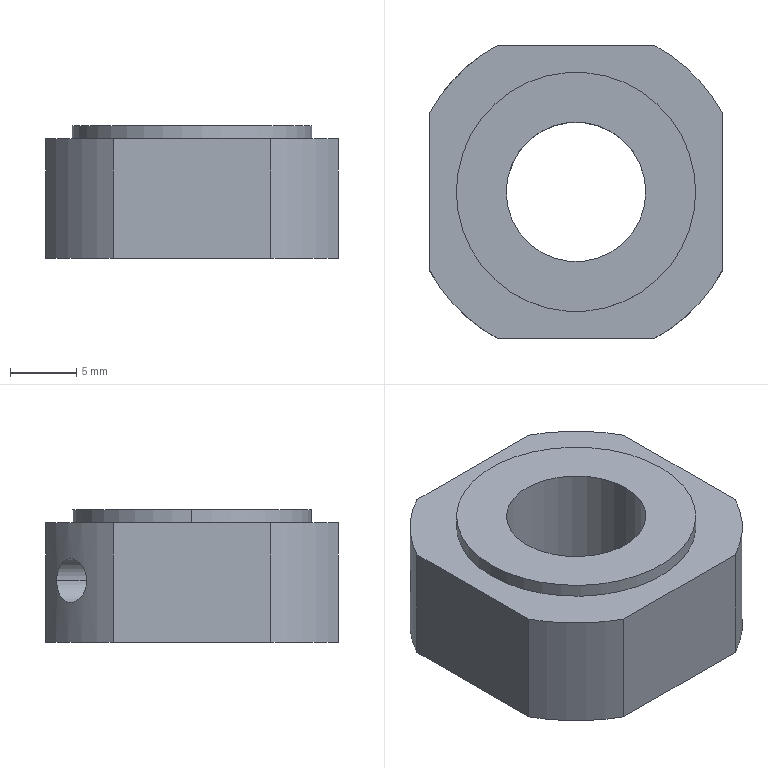Part | SolidWorks | features HoleWzd 2, 3DProfileFeature 1, Extrusion 1, ICE 1 | 1 solid | 17 faces | box 22 x 22 x 10 mm | volume 3311 mm3 | cylinder 10 | plane 7 | commonest cylinder face diameters 25 x4 3.3 x2 10.5 x2 18 x2
STEP:
#1=CARTESIAN_POINT('',(-5.25,0.,0.));
#2=VERTEX_POINT('',#1);
#3=CARTESIAN_POINT('',(5.25,0.,0.));
#4=VERTEX_POINT('',#3);
#5=CARTESIAN_POINT('',(0.,0.,0.));
#6=DIRECTION('',(0.,0.,1.));
#7=DIRECTION('',(1.,0.,0.));
#8=AXIS2_PLACEMENT_3D('',#5,#6,#7);
#9=CIRCLE('',#8,5.25);
#10=EDGE_CURVE('',#2,#4,#9,.T.);
#11=ORIENTED_EDGE('',*,*,#10,.F.);
#12=CARTESIAN_POINT('',(-5.25,0.,10.));
#13=VERTEX_POINT('',#12);
#14=CARTESIAN_POINT('',(-5.25,0.,10.));
#15=DIRECTION('',(0.,0.,1.));
#16=VECTOR('',#15,1000.);
#17=LINE('',#14,#16);
#18=EDGE_CURVE('',#2,#13,#17,.T.);
#19=ORIENTED_EDGE('',*,*,#18,.T.);
#20=CARTESIAN_POINT('',(5.25,0.,10.));
#21=VERTEX_POINT('',#20);
#22=CARTESIAN_POINT('',(0.,0.,10.));
#23=DIRECTION('',(0.,0.,1.));
#24=DIRECTION('',(1.,0.,0.));
#25=AXIS2_PLACEMENT_3D('',#22,#23,#24);
#26=CIRCLE('',#25,5.25);
#27=EDGE_CURVE('',#13,#21,#26,.T.);
#28=ORIENTED_EDGE('',*,*,#27,.T.);
#29=CARTESIAN_POINT('',(5.25,0.,10.));
#30=DIRECTION('',(0.,0.,1.));
#31=VECTOR('',#30,1000.);
#32=LINE('',#29,#31);
#33=EDGE_CURVE('',#4,#21,#32,.T.);
#34=ORIENTED_EDGE('',*,*,#33,.F.);
#35=EDGE_LOOP('',(#11,#19,#28,#34));
#36=FACE_OUTER_BOUND('',#35,.T.);
#37=CARTESIAN_POINT('',(0.,0.,10.));
#38=DIRECTION('',(0.,0.,1.));
#39=DIRECTION('',(1.,0.,0.));
#40=AXIS2_PLACEMENT_3D('',#37,#38,#39);
#41=CYLINDRICAL_SURFACE('',#40,5.25);
#42=ADVANCED_FACE('',(#36),#41,.F.);
#43=CARTESIAN_POINT('',(-4.609,2.514,4.65));
#44=VERTEX_POINT('',#43);
#45=CARTESIAN_POINT('',(-2.198,4.768,4.65));
#46=VERTEX_POINT('',#45);
#47=CARTESIAN_POINT('',(-4.609,2.514,4.65));
#48=CARTESIAN_POINT('',(-4.609,2.514,4.54));
#49=CARTESIAN_POINT('',(-4.603,2.525,4.432));
#50=CARTESIAN_POINT('',(-4.582,2.563,4.22));
#51=CARTESIAN_POINT('',(-4.565,2.593,4.115));
#52=CARTESIAN_POINT('',(-4.522,2.668,3.916));
#53=CARTESIAN_POINT('',(-4.495,2.713,3.821));
#54=CARTESIAN_POINT('',(-4.429,2.819,3.642));
#55=CARTESIAN_POINT('',(-4.391,2.879,3.558));
#56=CARTESIAN_POINT('',(-4.261,3.072,3.332));
#57=CARTESIAN_POINT('',(-4.15,3.221,3.209));
#58=CARTESIAN_POINT('',(-3.958,3.451,3.085));
#59=CARTESIAN_POINT('',(-3.888,3.53,3.053));
#60=CARTESIAN_POINT('',(-3.741,3.685,3.01));
#61=CARTESIAN_POINT('',(-3.665,3.761,3.));
#62=CARTESIAN_POINT('',(-3.506,3.909,3.));
#63=CARTESIAN_POINT('',(-3.423,3.982,3.01));
#64=CARTESIAN_POINT('',(-3.259,4.117,3.053));
#65=CARTESIAN_POINT('',(-3.177,4.181,3.084));
#66=CARTESIAN_POINT('',(-2.932,4.359,3.21));
#67=CARTESIAN_POINT('',(-2.777,4.458,3.331));
#68=CARTESIAN_POINT('',(-2.575,4.576,3.56));
#69=CARTESIAN_POINT('',(-2.514,4.61,3.642));
#70=CARTESIAN_POINT('',(-2.404,4.667,3.82));
#71=CARTESIAN_POINT('',(-2.356,4.692,3.917));
#72=CARTESIAN_POINT('',(-2.279,4.73,4.116));
#73=CARTESIAN_POINT('',(-2.249,4.744,4.219));
#74=CARTESIAN_POINT('',(-2.208,4.763,4.432));
#75=CARTESIAN_POINT('',(-2.198,4.768,4.541));
#76=CARTESIAN_POINT('',(-2.198,4.768,4.65));
#77=B_SPLINE_CURVE_WITH_KNOTS('',3,(#47,#48,#49,#50,#51,#52,#53,#54,#55,#56,#57,#58,#59,#60,#61,#62,#63,#64,#65,#66,#67,#68,#69,#70,#71,#72,#73,#74,#75,#76),.UNSPECIFIED.,.F.,.F.,(4,2,2,2,2,2,2,2,2,2,2,2,2,2,4),(0.,0.0003245,0.000649,0.0009734,0.001298,0.001947,0.002271,0.002596,0.00292,0.003245,0.003894,0.004218,0.004543,0.004867,0.005192),.UNSPECIFIED.);
#78=EDGE_CURVE('',#44,#46,#77,.T.);
#79=ORIENTED_EDGE('',*,*,#78,.T.);
#80=CARTESIAN_POINT('',(-7.255,10.179,4.65));
#81=VERTEX_POINT('',#80);
#82=CARTESIAN_POINT('',(-7.33,10.259,4.65));
#83=DIRECTION('',(-0.6828,0.7306,0.));
#84=VECTOR('',#83,1000.);
#85=LINE('',#82,#84);
#86=EDGE_CURVE('',#46,#81,#85,.T.);
#87=ORIENTED_EDGE('',*,*,#86,.T.);
#88=CARTESIAN_POINT('',(-9.666,7.926,4.65));
#89=VERTEX_POINT('',#88);
#90=CARTESIAN_POINT('',(-9.666,7.926,4.65));
#91=CARTESIAN_POINT('',(-9.666,7.926,4.54));
#92=CARTESIAN_POINT('',(-9.659,7.934,4.433));
#93=CARTESIAN_POINT('',(-9.632,7.967,4.222));
#94=CARTESIAN_POINT('',(-9.612,7.991,4.117));
#95=CARTESIAN_POINT('',(-9.558,8.055,3.917));
#96=CARTESIAN_POINT('',(-9.525,8.094,3.823));
#97=CARTESIAN_POINT('',(-9.447,8.186,3.643));
#98=CARTESIAN_POINT('',(-9.401,8.239,3.559));
#99=CARTESIAN_POINT('',(-9.249,8.41,3.331));
#100=CARTESIAN_POINT('',(-9.124,8.546,3.208));
#101=CARTESIAN_POINT('',(-8.848,8.832,3.043));
#102=CARTESIAN_POINT('',(-8.693,8.985,3.));
#103=CARTESIAN_POINT('',(-8.457,9.205,3.));
#104=CARTESIAN_POINT('',(-8.376,9.279,3.01));
#105=CARTESIAN_POINT('',(-8.218,9.42,3.053));
#106=CARTESIAN_POINT('',(-8.14,9.487,3.084));
#107=CARTESIAN_POINT('',(-7.987,9.616,3.166));
#108=CARTESIAN_POINT('',(-7.912,9.677,3.218));
#109=CARTESIAN_POINT('',(-7.773,9.79,3.338));
#110=CARTESIAN_POINT('',(-7.707,9.842,3.406));
#111=CARTESIAN_POINT('',(-7.585,9.936,3.56));
#112=CARTESIAN_POINT('',(-7.53,9.978,3.643));
#113=CARTESIAN_POINT('',(-7.434,10.049,3.822));
#114=CARTESIAN_POINT('',(-7.392,10.08,3.918));
#115=CARTESIAN_POINT('',(-7.324,10.129,4.118));
#116=CARTESIAN_POINT('',(-7.299,10.148,4.221));
#117=CARTESIAN_POINT('',(-7.264,10.173,4.432));
#118=CARTESIAN_POINT('',(-7.255,10.179,4.542));
#119=CARTESIAN_POINT('',(-7.255,10.179,4.65));
#120=B_SPLINE_CURVE_WITH_KNOTS('',3,(#90,#91,#92,#93,#94,#95,#96,#97,#98,#99,#100,#101,#102,#103,#104,#105,#106,#107,#108,#109,#110,#111,#112,#113,#114,#115,#116,#117,#118,#119),.UNSPECIFIED.,.F.,.F.,(4,2,2,2,2,2,2,2,2,2,2,2,2,2,4),(0.,0.0003228,0.0006455,0.0009683,0.001291,0.001937,0.002582,0.002905,0.003228,0.00355,0.003873,0.004196,0.004519,0.004842,0.005164),.UNSPECIFIED.);
#121=EDGE_CURVE('',#89,#81,#120,.T.);
#122=ORIENTED_EDGE('',*,*,#121,.F.);
#123=CARTESIAN_POINT('',(-9.741,8.005,4.65));
#124=DIRECTION('',(-0.6828,0.7306,0.));
#125=VECTOR('',#124,1000.);
#126=LINE('',#123,#125);
#127=EDGE_CURVE('',#44,#89,#126,.T.);
#128=ORIENTED_EDGE('',*,*,#127,.F.);
#129=EDGE_LOOP('',(#79,#87,#122,#128));
#130=FACE_OUTER_BOUND('',#129,.T.);
#131=CARTESIAN_POINT('',(-8.535,9.132,4.65));
#132=DIRECTION('',(-0.6828,0.7306,0.));
#133=DIRECTION('',(-0.7306,-0.6828,0.));
#134=AXIS2_PLACEMENT_3D('',#131,#132,#133);
#135=CYLINDRICAL_SURFACE('',#134,1.65);
#136=ADVANCED_FACE('',(#130),#135,.F.);
#137=CARTESIAN_POINT('',(9.,0.,9.));
#138=VERTEX_POINT('',#137);
#139=CARTESIAN_POINT('',(-9.,0.,9.));
#140=VERTEX_POINT('',#139);
#141=CARTESIAN_POINT('',(0.,0.,9.));
#142=DIRECTION('',(0.,0.,1.));
#143=DIRECTION('',(1.,0.,0.));
#144=AXIS2_PLACEMENT_3D('',#141,#142,#143);
#145=CIRCLE('',#144,9.);
#146=EDGE_CURVE('',#138,#140,#145,.T.);
#147=ORIENTED_EDGE('',*,*,#146,.T.);
#148=CARTESIAN_POINT('',(-9.,0.,10.));
#149=VERTEX_POINT('',#148);
#150=CARTESIAN_POINT('',(-9.,0.,9.));
#151=DIRECTION('',(0.,0.,1.));
#152=VECTOR('',#151,1000.);
#153=LINE('',#150,#152);
#154=EDGE_CURVE('',#140,#149,#153,.T.);
#155=ORIENTED_EDGE('',*,*,#154,.T.);
#156=CARTESIAN_POINT('',(9.,0.,10.));
#157=VERTEX_POINT('',#156);
#158=CARTESIAN_POINT('',(0.,0.,10.));
#159=DIRECTION('',(0.,0.,1.));
#160=DIRECTION('',(1.,0.,0.));
#161=AXIS2_PLACEMENT_3D('',#158,#159,#160);
#162=CIRCLE('',#161,9.);
#163=EDGE_CURVE('',#157,#149,#162,.T.);
#164=ORIENTED_EDGE('',*,*,#163,.F.);
#165=CARTESIAN_POINT('',(9.,0.,9.));
#166=DIRECTION('',(0.,0.,1.));
#167=VECTOR('',#166,1000.);
#168=LINE('',#165,#167);
#169=EDGE_CURVE('',#138,#157,#168,.T.);
#170=ORIENTED_EDGE('',*,*,#169,.F.);
#171=EDGE_LOOP('',(#147,#155,#164,#170));
#172=FACE_OUTER_BOUND('',#171,.T.);
#173=CARTESIAN_POINT('',(0.,0.,9.));
#174=DIRECTION('',(0.,0.,1.));
#175=DIRECTION('',(1.,0.,0.));
#176=AXIS2_PLACEMENT_3D('',#173,#174,#175);
#177=CYLINDRICAL_SURFACE('',#176,9.);
#178=ADVANCED_FACE('',(#172),#177,.T.);
#179=CARTESIAN_POINT('',(5.937,-11.,9.));
#180=VERTEX_POINT('',#179);
#181=CARTESIAN_POINT('',(11.,-5.937,9.));
#182=VERTEX_POINT('',#181);
#183=CARTESIAN_POINT('',(0.,0.,9.));
#184=DIRECTION('',(0.,0.,1.));
#185=DIRECTION('',(1.,0.,0.));
#186=AXIS2_PLACEMENT_3D('',#183,#184,#185);
#187=CIRCLE('',#186,12.5);
#188=EDGE_CURVE('',#180,#182,#187,.T.);
#189=ORIENTED_EDGE('',*,*,#188,.F.);
#190=CARTESIAN_POINT('',(5.937,-11.,0.));
#191=VERTEX_POINT('',#190);
#192=CARTESIAN_POINT('',(5.937,-11.,10.));
#193=DIRECTION('',(0.,0.,-1.));
#194=VECTOR('',#193,1000.);
#195=LINE('',#192,#194);
#196=EDGE_CURVE('',#180,#191,#195,.T.);
#197=ORIENTED_EDGE('',*,*,#196,.T.);
#198=CARTESIAN_POINT('',(11.,-5.937,0.));
#199=VERTEX_POINT('',#198);
#200=CARTESIAN_POINT('',(0.,0.,0.));
#201=DIRECTION('',(0.,0.,1.));
#202=DIRECTION('',(1.,0.,0.));
#203=AXIS2_PLACEMENT_3D('',#200,#201,#202);
#204=CIRCLE('',#203,12.5);
#205=EDGE_CURVE('',#191,#199,#204,.T.);
#206=ORIENTED_EDGE('',*,*,#205,.T.);
#207=CARTESIAN_POINT('',(11.,-5.937,10.));
#208=DIRECTION('',(0.,0.,-1.));
#209=VECTOR('',#208,1000.);
#210=LINE('',#207,#209);
#211=EDGE_CURVE('',#182,#199,#210,.T.);
#212=ORIENTED_EDGE('',*,*,#211,.F.);
#213=EDGE_LOOP('',(#189,#197,#206,#212));
#214=FACE_OUTER_BOUND('',#213,.T.);
#215=CARTESIAN_POINT('',(0.,0.,10.));
#216=DIRECTION('',(0.,0.,-1.));
#217=DIRECTION('',(-1.,0.,0.));
#218=AXIS2_PLACEMENT_3D('',#215,#216,#217);
#219=CYLINDRICAL_SURFACE('',#218,12.5);
#220=ADVANCED_FACE('',(#214),#219,.T.);
#221=CARTESIAN_POINT('',(11.,5.937,9.));
#222=VERTEX_POINT('',#221);
#223=CARTESIAN_POINT('',(11.,-5.937,9.));
#224=DIRECTION('',(0.,1.,0.));
#225=VECTOR('',#224,1000.);
#226=LINE('',#223,#225);
#227=EDGE_CURVE('',#182,#222,#226,.T.);
#228=ORIENTED_EDGE('',*,*,#227,.F.);
#229=ORIENTED_EDGE('',*,*,#211,.T.);
#230=CARTESIAN_POINT('',(11.,5.937,0.));
#231=VERTEX_POINT('',#230);
#232=CARTESIAN_POINT('',(11.,-5.937,0.));
#233=DIRECTION('',(0.,1.,0.));
#234=VECTOR('',#233,1000.);
#235=LINE('',#232,#234);
#236=EDGE_CURVE('',#199,#231,#235,.T.);
#237=ORIENTED_EDGE('',*,*,#236,.T.);
#238=CARTESIAN_POINT('',(11.,5.937,10.));
#239=DIRECTION('',(0.,0.,-1.));
#240=VECTOR('',#239,1000.);
#241=LINE('',#238,#240);
#242=EDGE_CURVE('',#222,#231,#241,.T.);
#243=ORIENTED_EDGE('',*,*,#242,.F.);
#244=EDGE_LOOP('',(#228,#229,#237,#243));
#245=FACE_OUTER_BOUND('',#244,.T.);
#246=CARTESIAN_POINT('',(11.,-5.937,10.));
#247=DIRECTION('',(-1.,0.,0.));
#248=DIRECTION('',(0.,0.,1.));
#249=AXIS2_PLACEMENT_3D('',#246,#247,#248);
#250=PLANE('',#249);
#251=ADVANCED_FACE('',(#245),#250,.F.);
#252=CARTESIAN_POINT('',(5.937,11.,9.));
#253=VERTEX_POINT('',#252);
#254=CARTESIAN_POINT('',(0.,0.,9.));
#255=DIRECTION('',(0.,0.,1.));
#256=DIRECTION('',(1.,0.,0.));
#257=AXIS2_PLACEMENT_3D('',#254,#255,#256);
#258=CIRCLE('',#257,12.5);
#259=EDGE_CURVE('',#222,#253,#258,.T.);
#260=ORIENTED_EDGE('',*,*,#259,.F.);
#261=ORIENTED_EDGE('',*,*,#242,.T.);
#262=CARTESIAN_POINT('',(5.937,11.,0.));
#263=VERTEX_POINT('',#262);
#264=CARTESIAN_POINT('',(0.,0.,0.));
#265=DIRECTION('',(0.,0.,1.));
#266=DIRECTION('',(1.,0.,0.));
#267=AXIS2_PLACEMENT_3D('',#264,#265,#266);
#268=CIRCLE('',#267,12.5);
#269=EDGE_CURVE('',#231,#263,#268,.T.);
#270=ORIENTED_EDGE('',*,*,#269,.T.);
#271=CARTESIAN_POINT('',(5.937,11.,10.));
#272=DIRECTION('',(0.,0.,-1.));
#273=VECTOR('',#272,1000.);
#274=LINE('',#271,#273);
#275=EDGE_CURVE('',#253,#263,#274,.T.);
#276=ORIENTED_EDGE('',*,*,#275,.F.);
#277=EDGE_LOOP('',(#260,#261,#270,#276));
#278=FACE_OUTER_BOUND('',#277,.T.);
#279=CARTESIAN_POINT('',(0.,0.,10.));
#280=DIRECTION('',(0.,0.,-1.));
#281=DIRECTION('',(-1.,0.,0.));
#282=AXIS2_PLACEMENT_3D('',#279,#280,#281);
#283=CYLINDRICAL_SURFACE('',#282,12.5);
#284=ADVANCED_FACE('',(#278),#283,.T.);
#285=CARTESIAN_POINT('',(-5.937,11.,9.));
#286=VERTEX_POINT('',#285);
#287=CARTESIAN_POINT('',(5.937,11.,9.));
#288=DIRECTION('',(-1.,0.,0.));
#289=VECTOR('',#288,1000.);
#290=LINE('',#287,#289);
#291=EDGE_CURVE('',#253,#286,#290,.T.);
#292=ORIENTED_EDGE('',*,*,#291,.F.);
#293=ORIENTED_EDGE('',*,*,#275,.T.);
#294=CARTESIAN_POINT('',(-5.937,11.,0.));
#295=VERTEX_POINT('',#294);
#296=CARTESIAN_POINT('',(5.937,11.,0.));
#297=DIRECTION('',(-1.,0.,0.));
#298=VECTOR('',#297,1000.);
#299=LINE('',#296,#298);
#300=EDGE_CURVE('',#263,#295,#299,.T.);
#301=ORIENTED_EDGE('',*,*,#300,.T.);
#302=CARTESIAN_POINT('',(-5.937,11.,10.));
#303=DIRECTION('',(0.,0.,-1.));
#304=VECTOR('',#303,1000.);
#305=LINE('',#302,#304);
#306=EDGE_CURVE('',#286,#295,#305,.T.);
#307=ORIENTED_EDGE('',*,*,#306,.F.);
#308=EDGE_LOOP('',(#292,#293,#301,#307));
#309=FACE_OUTER_BOUND('',#308,.T.);
#310=CARTESIAN_POINT('',(5.937,11.,10.));
#311=DIRECTION('',(0.,-1.,0.));
#312=DIRECTION('',(1.,0.,0.));
#313=AXIS2_PLACEMENT_3D('',#310,#311,#312);
#314=PLANE('',#313);
#315=ADVANCED_FACE('',(#309),#314,.F.);
#316=ORIENTED_EDGE('',*,*,#121,.T.);
#317=CARTESIAN_POINT('',(-7.255,10.179,4.65));
#318=CARTESIAN_POINT('',(-7.255,10.179,4.865));
#319=CARTESIAN_POINT('',(-7.291,10.154,5.082));
#320=CARTESIAN_POINT('',(-7.425,10.056,5.479));
#321=CARTESIAN_POINT('',(-7.524,9.983,5.663));
#322=CARTESIAN_POINT('',(-7.706,9.843,5.892));
#323=CARTESIAN_POINT('',(-7.772,9.79,5.961));
#324=CARTESIAN_POINT('',(-7.912,9.678,6.081));
#325=CARTESIAN_POINT('',(-7.986,9.617,6.132));
#326=CARTESIAN_POINT('',(-8.138,9.488,6.215));
#327=CARTESIAN_POINT('',(-8.218,9.42,6.247));
#328=CARTESIAN_POINT('',(-8.376,9.28,6.289));
#329=CARTESIAN_POINT('',(-8.455,9.207,6.3));
#330=CARTESIAN_POINT('',(-8.614,9.058,6.3));
#331=CARTESIAN_POINT('',(-8.692,8.984,6.289));
#332=CARTESIAN_POINT('',(-8.842,8.836,6.247));
#333=CARTESIAN_POINT('',(-8.916,8.761,6.215));
#334=CARTESIAN_POINT('',(-9.055,8.618,6.133));
#335=CARTESIAN_POINT('',(-9.12,8.549,6.082));
#336=CARTESIAN_POINT('',(-9.242,8.416,5.963));
#337=CARTESIAN_POINT('',(-9.299,8.353,5.893));
#338=CARTESIAN_POINT('',(-9.451,8.182,5.665));
#339=CARTESIAN_POINT('',(-9.532,8.087,5.481));
#340=CARTESIAN_POINT('',(-9.638,7.96,5.085));
#341=CARTESIAN_POINT('',(-9.666,7.926,4.868));
#342=CARTESIAN_POINT('',(-9.666,7.926,4.65));
#343=B_SPLINE_CURVE_WITH_KNOTS('',3,(#317,#318,#319,#320,#321,#322,#323,#324,#325,#326,#327,#328,#329,#330,#331,#332,#333,#334,#335,#336,#337,#338,#339,#340,#341,#342),.UNSPECIFIED.,.F.,.F.,(4,2,2,2,2,2,2,2,2,2,2,2,4),(0.005164,0.00581,0.006455,0.006778,0.0071,0.007423,0.007746,0.008068,0.008391,0.008714,0.009037,0.009682,0.01033),.UNSPECIFIED.);
#344=EDGE_CURVE('',#81,#89,#343,.T.);
#345=ORIENTED_EDGE('',*,*,#344,.T.);
#346=EDGE_LOOP('',(#316,#345));
#347=FACE_BOUND('',#346,.T.);
#348=CARTESIAN_POINT('',(-11.,5.937,9.));
#349=VERTEX_POINT('',#348);
#350=CARTESIAN_POINT('',(0.,0.,9.));
#351=DIRECTION('',(0.,0.,1.));
#352=DIRECTION('',(1.,0.,0.));
#353=AXIS2_PLACEMENT_3D('',#350,#351,#352);
#354=CIRCLE('',#353,12.5);
#355=EDGE_CURVE('',#286,#349,#354,.T.);
#356=ORIENTED_EDGE('',*,*,#355,.F.);
#357=ORIENTED_EDGE('',*,*,#306,.T.);
#358=CARTESIAN_POINT('',(-11.,5.937,0.));
#359=VERTEX_POINT('',#358);
#360=CARTESIAN_POINT('',(0.,0.,0.));
#361=DIRECTION('',(0.,0.,1.));
#362=DIRECTION('',(1.,0.,0.));
#363=AXIS2_PLACEMENT_3D('',#360,#361,#362);
#364=CIRCLE('',#363,12.5);
#365=EDGE_CURVE('',#295,#359,#364,.T.);
#366=ORIENTED_EDGE('',*,*,#365,.T.);
#367=CARTESIAN_POINT('',(-11.,5.937,10.));
#368=DIRECTION('',(0.,0.,-1.));
#369=VECTOR('',#368,1000.);
#370=LINE('',#367,#369);
#371=EDGE_CURVE('',#349,#359,#370,.T.);
#372=ORIENTED_EDGE('',*,*,#371,.F.);
#373=EDGE_LOOP('',(#356,#357,#366,#372));
#374=FACE_OUTER_BOUND('',#373,.T.);
#375=CARTESIAN_POINT('',(0.,0.,10.));
#376=DIRECTION('',(0.,0.,-1.));
#377=DIRECTION('',(-1.,0.,0.));
#378=AXIS2_PLACEMENT_3D('',#375,#376,#377);
#379=CYLINDRICAL_SURFACE('',#378,12.5);
#380=ADVANCED_FACE('',(#347,#374),#379,.T.);
#381=CARTESIAN_POINT('',(-11.,-5.937,9.));
#382=VERTEX_POINT('',#381);
#383=CARTESIAN_POINT('',(-11.,5.937,9.));
#384=DIRECTION('',(0.,-1.,0.));
#385=VECTOR('',#384,1000.);
#386=LINE('',#383,#385);
#387=EDGE_CURVE('',#349,#382,#386,.T.);
#388=ORIENTED_EDGE('',*,*,#387,.F.);
#389=ORIENTED_EDGE('',*,*,#371,.T.);
#390=CARTESIAN_POINT('',(-11.,-5.937,0.));
#391=VERTEX_POINT('',#390);
#392=CARTESIAN_POINT('',(-11.,5.937,0.));
#393=DIRECTION('',(0.,-1.,0.));
#394=VECTOR('',#393,1000.);
#395=LINE('',#392,#394);
#396=EDGE_CURVE('',#359,#391,#395,.T.);
#397=ORIENTED_EDGE('',*,*,#396,.T.);
#398=CARTESIAN_POINT('',(-11.,-5.937,10.));
#399=DIRECTION('',(0.,0.,-1.));
#400=VECTOR('',#399,1000.);
#401=LINE('',#398,#400);
#402=EDGE_CURVE('',#382,#391,#401,.T.);
#403=ORIENTED_EDGE('',*,*,#402,.F.);
#404=EDGE_LOOP('',(#388,#389,#397,#403));
#405=FACE_OUTER_BOUND('',#404,.T.);
#406=CARTESIAN_POINT('',(-11.,5.937,10.));
#407=DIRECTION('',(1.,0.,0.));
#408=DIRECTION('',(0.,1.,0.));
#409=AXIS2_PLACEMENT_3D('',#406,#407,#408);
#410=PLANE('',#409);
#411=ADVANCED_FACE('',(#405),#410,.F.);
#412=CARTESIAN_POINT('',(-5.937,-11.,9.));
#413=VERTEX_POINT('',#412);
#414=CARTESIAN_POINT('',(0.,0.,9.));
#415=DIRECTION('',(0.,0.,1.));
#416=DIRECTION('',(1.,0.,0.));
#417=AXIS2_PLACEMENT_3D('',#414,#415,#416);
#418=CIRCLE('',#417,12.5);
#419=EDGE_CURVE('',#382,#413,#418,.T.);
#420=ORIENTED_EDGE('',*,*,#419,.F.);
#421=ORIENTED_EDGE('',*,*,#402,.T.);
#422=CARTESIAN_POINT('',(-5.937,-11.,0.));
#423=VERTEX_POINT('',#422);
#424=CARTESIAN_POINT('',(0.,0.,0.));
#425=DIRECTION('',(0.,0.,1.));
#426=DIRECTION('',(1.,0.,0.));
#427=AXIS2_PLACEMENT_3D('',#424,#425,#426);
#428=CIRCLE('',#427,12.5);
#429=EDGE_CURVE('',#391,#423,#428,.T.);
#430=ORIENTED_EDGE('',*,*,#429,.T.);
#431=CARTESIAN_POINT('',(-5.937,-11.,10.));
#432=DIRECTION('',(0.,0.,-1.));
#433=VECTOR('',#432,1000.);
#434=LINE('',#431,#433);
#435=EDGE_CURVE('',#413,#423,#434,.T.);
#436=ORIENTED_EDGE('',*,*,#435,.F.);
#437=EDGE_LOOP('',(#420,#421,#430,#436));
#438=FACE_OUTER_BOUND('',#437,.T.);
#439=CARTESIAN_POINT('',(0.,0.,10.));
#440=DIRECTION('',(0.,0.,-1.));
#441=DIRECTION('',(-1.,0.,0.));
#442=AXIS2_PLACEMENT_3D('',#439,#440,#441);
#443=CYLINDRICAL_SURFACE('',#442,12.5);
#444=ADVANCED_FACE('',(#438),#443,.T.);
#445=CARTESIAN_POINT('',(-5.937,-11.,9.));
#446=DIRECTION('',(1.,0.,0.));
#447=VECTOR('',#446,1000.);
#448=LINE('',#445,#447);
#449=EDGE_CURVE('',#413,#180,#448,.T.);
#450=ORIENTED_EDGE('',*,*,#449,.F.);
#451=ORIENTED_EDGE('',*,*,#435,.T.);
#452=CARTESIAN_POINT('',(-5.937,-11.,0.));
#453=DIRECTION('',(1.,0.,0.));
#454=VECTOR('',#453,1000.);
#455=LINE('',#452,#454);
#456=EDGE_CURVE('',#423,#191,#455,.T.);
#457=ORIENTED_EDGE('',*,*,#456,.T.);
#458=ORIENTED_EDGE('',*,*,#196,.F.);
#459=EDGE_LOOP('',(#450,#451,#457,#458));
#460=FACE_OUTER_BOUND('',#459,.T.);
#461=CARTESIAN_POINT('',(-5.937,-11.,10.));
#462=DIRECTION('',(0.,1.,0.));
#463=DIRECTION('',(-1.,0.,0.));
#464=AXIS2_PLACEMENT_3D('',#461,#462,#463);
#465=PLANE('',#464);
#466=ADVANCED_FACE('',(#460),#465,.F.);
#467=CARTESIAN_POINT('',(0.,0.,0.));
#468=DIRECTION('',(0.,0.,1.));
#469=DIRECTION('',(1.,0.,0.));
#470=AXIS2_PLACEMENT_3D('',#467,#468,#469);
#471=CIRCLE('',#470,5.25);
#472=EDGE_CURVE('',#4,#2,#471,.T.);
#473=ORIENTED_EDGE('',*,*,#472,.T.);
#474=ORIENTED_EDGE('',*,*,#10,.T.);
#475=EDGE_LOOP('',(#473,#474));
#476=FACE_BOUND('',#475,.T.);
#477=ORIENTED_EDGE('',*,*,#205,.F.);
#478=ORIENTED_EDGE('',*,*,#456,.F.);
#479=ORIENTED_EDGE('',*,*,#429,.F.);
#480=ORIENTED_EDGE('',*,*,#396,.F.);
#481=ORIENTED_EDGE('',*,*,#365,.F.);
#482=ORIENTED_EDGE('',*,*,#300,.F.);
#483=ORIENTED_EDGE('',*,*,#269,.F.);
#484=ORIENTED_EDGE('',*,*,#236,.F.);
#485=EDGE_LOOP('',(#477,#478,#479,#480,#481,#482,#483,#484));
#486=FACE_OUTER_BOUND('',#485,.T.);
#487=CARTESIAN_POINT('',(0.,0.,0.));
#488=DIRECTION('',(0.,0.,1.));
#489=DIRECTION('',(1.,0.,0.));
#490=AXIS2_PLACEMENT_3D('',#487,#488,#489);
#491=PLANE('',#490);
#492=ADVANCED_FACE('',(#476,#486),#491,.F.);
#493=ORIENTED_EDGE('',*,*,#146,.F.);
#494=CARTESIAN_POINT('',(0.,0.,9.));
#495=DIRECTION('',(0.,0.,1.));
#496=DIRECTION('',(1.,0.,0.));
#497=AXIS2_PLACEMENT_3D('',#494,#495,#496);
#498=CIRCLE('',#497,9.);
#499=EDGE_CURVE('',#140,#138,#498,.T.);
#500=ORIENTED_EDGE('',*,*,#499,.F.);
#501=EDGE_LOOP('',(#493,#500));
#502=FACE_BOUND('',#501,.T.);
#503=ORIENTED_EDGE('',*,*,#188,.T.);
#504=ORIENTED_EDGE('',*,*,#227,.T.);
#505=ORIENTED_EDGE('',*,*,#259,.T.);
#506=ORIENTED_EDGE('',*,*,#291,.T.);
#507=ORIENTED_EDGE('',*,*,#355,.T.);
#508=ORIENTED_EDGE('',*,*,#387,.T.);
#509=ORIENTED_EDGE('',*,*,#419,.T.);
#510=ORIENTED_EDGE('',*,*,#449,.T.);
#511=EDGE_LOOP('',(#503,#504,#505,#506,#507,#508,#509,#510));
#512=FACE_OUTER_BOUND('',#511,.T.);
#513=CARTESIAN_POINT('',(0.,0.,9.));
#514=DIRECTION('',(0.,0.,1.));
#515=DIRECTION('',(1.,0.,0.));
#516=AXIS2_PLACEMENT_3D('',#513,#514,#515);
#517=PLANE('',#516);
#518=ADVANCED_FACE('',(#502,#512),#517,.T.);
#519=ORIENTED_EDGE('',*,*,#154,.F.);
#520=ORIENTED_EDGE('',*,*,#499,.T.);
#521=ORIENTED_EDGE('',*,*,#169,.T.);
#522=CARTESIAN_POINT('',(0.,0.,10.));
#523=DIRECTION('',(0.,0.,1.));
#524=DIRECTION('',(1.,0.,0.));
#525=AXIS2_PLACEMENT_3D('',#522,#523,#524);
#526=CIRCLE('',#525,9.);
#527=EDGE_CURVE('',#149,#157,#526,.T.);
#528=ORIENTED_EDGE('',*,*,#527,.F.);
#529=EDGE_LOOP('',(#519,#520,#521,#528));
#530=FACE_OUTER_BOUND('',#529,.T.);
#531=CARTESIAN_POINT('',(0.,0.,9.));
#532=DIRECTION('',(0.,0.,1.));
#533=DIRECTION('',(1.,0.,0.));
#534=AXIS2_PLACEMENT_3D('',#531,#532,#533);
#535=CYLINDRICAL_SURFACE('',#534,9.);
#536=ADVANCED_FACE('',(#530),#535,.T.);
#537=CARTESIAN_POINT('',(0.,0.,10.));
#538=DIRECTION('',(0.,0.,1.));
#539=DIRECTION('',(1.,0.,0.));
#540=AXIS2_PLACEMENT_3D('',#537,#538,#539);
#541=CIRCLE('',#540,5.25);
#542=EDGE_CURVE('',#21,#13,#541,.T.);
#543=ORIENTED_EDGE('',*,*,#542,.F.);
#544=ORIENTED_EDGE('',*,*,#27,.F.);
#545=EDGE_LOOP('',(#543,#544));
#546=FACE_BOUND('',#545,.T.);
#547=ORIENTED_EDGE('',*,*,#163,.T.);
#548=ORIENTED_EDGE('',*,*,#527,.T.);
#549=EDGE_LOOP('',(#547,#548));
#550=FACE_OUTER_BOUND('',#549,.T.);
#551=CARTESIAN_POINT('',(0.,0.,10.));
#552=DIRECTION('',(0.,0.,1.));
#553=DIRECTION('',(1.,0.,0.));
#554=AXIS2_PLACEMENT_3D('',#551,#552,#553);
#555=PLANE('',#554);
#556=ADVANCED_FACE('',(#546,#550),#555,.T.);
#557=ORIENTED_EDGE('',*,*,#86,.F.);
#558=CARTESIAN_POINT('',(-2.198,4.768,4.65));
#559=CARTESIAN_POINT('',(-2.198,4.768,4.866));
#560=CARTESIAN_POINT('',(-2.24,4.749,5.084));
#561=CARTESIAN_POINT('',(-2.356,4.692,5.382));
#562=CARTESIAN_POINT('',(-2.404,4.667,5.479));
#563=CARTESIAN_POINT('',(-2.514,4.609,5.657));
#564=CARTESIAN_POINT('',(-2.575,4.576,5.74));
#565=CARTESIAN_POINT('',(-2.778,4.458,5.968));
#566=CARTESIAN_POINT('',(-2.932,4.36,6.089));
#567=CARTESIAN_POINT('',(-3.177,4.181,6.215));
#568=CARTESIAN_POINT('',(-3.259,4.117,6.246));
#569=CARTESIAN_POINT('',(-3.423,3.982,6.289));
#570=CARTESIAN_POINT('',(-3.505,3.91,6.3));
#571=CARTESIAN_POINT('',(-3.664,3.761,6.3));
#572=CARTESIAN_POINT('',(-3.741,3.685,6.289));
#573=CARTESIAN_POINT('',(-3.887,3.53,6.246));
#574=CARTESIAN_POINT('',(-3.957,3.451,6.214));
#575=CARTESIAN_POINT('',(-4.15,3.221,6.09));
#576=CARTESIAN_POINT('',(-4.261,3.071,5.968));
#577=CARTESIAN_POINT('',(-4.391,2.879,5.741));
#578=CARTESIAN_POINT('',(-4.43,2.819,5.657));
#579=CARTESIAN_POINT('',(-4.495,2.713,5.478));
#580=CARTESIAN_POINT('',(-4.522,2.668,5.384));
#581=CARTESIAN_POINT('',(-4.565,2.593,5.185));
#582=CARTESIAN_POINT('',(-4.582,2.564,5.079));
#583=CARTESIAN_POINT('',(-4.603,2.525,4.867));
#584=CARTESIAN_POINT('',(-4.609,2.514,4.759));
#585=CARTESIAN_POINT('',(-4.609,2.514,4.65));
#586=B_SPLINE_CURVE_WITH_KNOTS('',3,(#558,#559,#560,#561,#562,#563,#564,#565,#566,#567,#568,#569,#570,#571,#572,#573,#574,#575,#576,#577,#578,#579,#580,#581,#582,#583,#584,#585),.UNSPECIFIED.,.F.,.F.,(4,2,2,2,2,2,2,2,2,2,2,2,2,4),(0.005192,0.00584,0.006165,0.006489,0.007138,0.007462,0.007787,0.008111,0.008436,0.009084,0.009409,0.009733,0.01006,0.01038),.UNSPECIFIED.);
#587=EDGE_CURVE('',#46,#44,#586,.T.);
#588=ORIENTED_EDGE('',*,*,#587,.T.);
#589=ORIENTED_EDGE('',*,*,#127,.T.);
#590=ORIENTED_EDGE('',*,*,#344,.F.);
#591=EDGE_LOOP('',(#557,#588,#589,#590));
#592=FACE_OUTER_BOUND('',#591,.T.);
#593=CARTESIAN_POINT('',(-8.535,9.132,4.65));
#594=DIRECTION('',(-0.6828,0.7306,0.));
#595=DIRECTION('',(-0.7306,-0.6828,0.));
#596=AXIS2_PLACEMENT_3D('',#593,#594,#595);
#597=CYLINDRICAL_SURFACE('',#596,1.65);
#598=ADVANCED_FACE('',(#592),#597,.F.);
#599=ORIENTED_EDGE('',*,*,#18,.F.);
#600=ORIENTED_EDGE('',*,*,#472,.F.);
#601=ORIENTED_EDGE('',*,*,#33,.T.);
#602=ORIENTED_EDGE('',*,*,#542,.T.);
#603=EDGE_LOOP('',(#599,#600,#601,#602));
#604=FACE_OUTER_BOUND('',#603,.T.);
#605=ORIENTED_EDGE('',*,*,#78,.F.);
#606=ORIENTED_EDGE('',*,*,#587,.F.);
#607=EDGE_LOOP('',(#605,#606));
#608=FACE_BOUND('',#607,.T.);
#609=CARTESIAN_POINT('',(0.,0.,10.));
#610=DIRECTION('',(0.,0.,1.));
#611=DIRECTION('',(1.,0.,0.));
#612=AXIS2_PLACEMENT_3D('',#609,#610,#611);
#613=CYLINDRICAL_SURFACE('',#612,5.25);
#614=ADVANCED_FACE('',(#604,#608),#613,.F.);
#615=CLOSED_SHELL('',(#42,#136,#178,#220,#251,#284,#315,#380,#411,#444,#466,#492,#518,#536,#556,#598,#614));
#616=MANIFOLD_SOLID_BREP('',#615);
#617=CARTESIAN_POINT('',(0.,0.,0.));
#618=DIRECTION('',(0.,0.,1.));
#619=DIRECTION('',(1.,0.,0.));
#620=AXIS2_PLACEMENT_3D('',#617,#618,#619);
#621=(LENGTH_UNIT()NAMED_UNIT(*)SI_UNIT(.MILLI.,.METRE.));
#622=UNCERTAINTY_MEASURE_WITH_UNIT(LENGTH_MEASURE(0.00001),#621,'','');
#623=(NAMED_UNIT(*)PLANE_ANGLE_UNIT()SI_UNIT($,.RADIAN.));
#624=(NAMED_UNIT(*)SI_UNIT($,.STERADIAN.)SOLID_ANGLE_UNIT());
#625=(GEOMETRIC_REPRESENTATION_CONTEXT(3)GLOBAL_UNCERTAINTY_ASSIGNED_CONTEXT((#622))GLOBAL_UNIT_ASSIGNED_CONTEXT((#621,#623,#624))REPRESENTATION_CONTEXT('',''));
#626=ADVANCED_BREP_SHAPE_REPRESENTATION('',(#616,#620),#625);